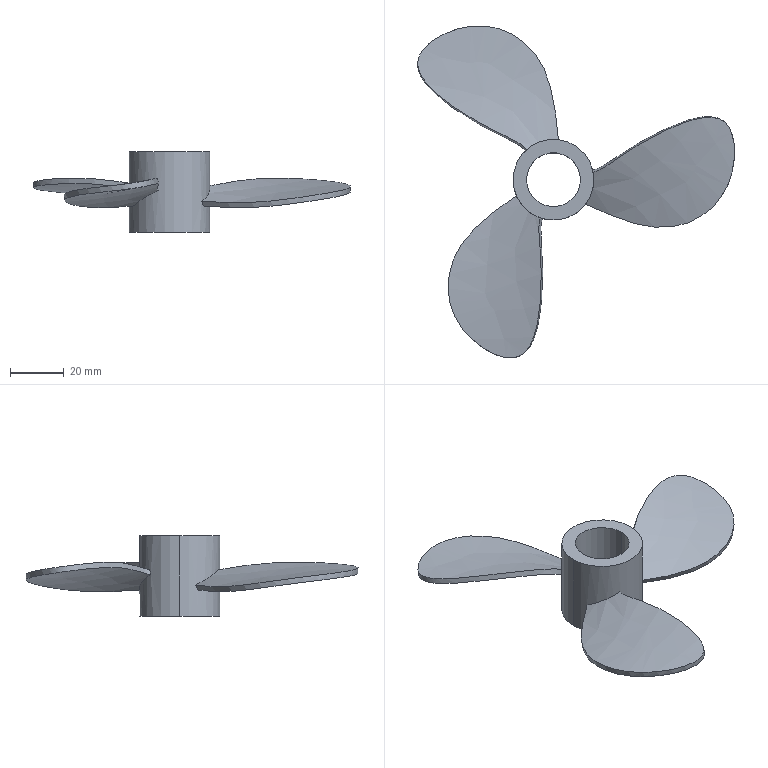Part | SolidWorks | features BlendRefSurface 1, CirPattern 1, CombineBodies 1, Extrusion 1, ICE 1, Thicken 1, TrimRefSurface 1 | 1 solid | 15 faces | box 117.735 x 123.352 x 30 mm | volume 21277 mm3 | spline 9 | cylinder 4 | plane 2 | commonest cylinder face diameters 20 x2 30 x2